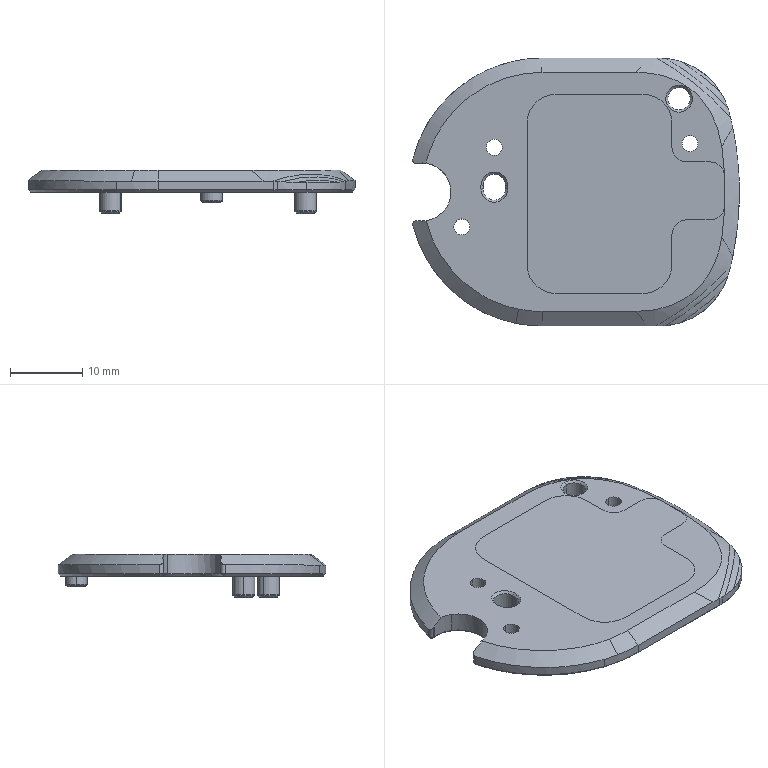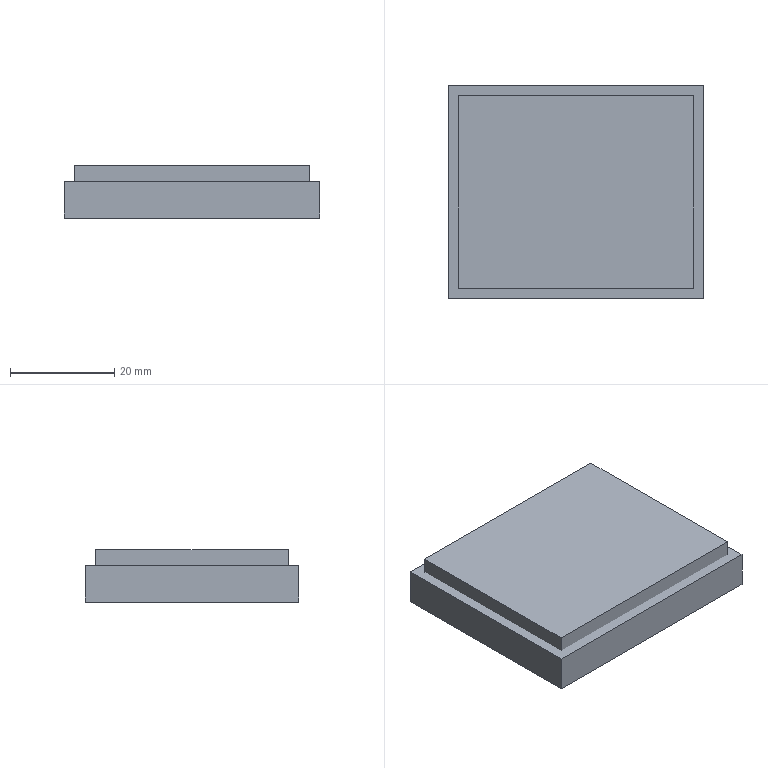CAM job | NX | 3-axis milling | part box 45.101 x 36.973 x 6 mm | stock box 49.101 x 40.973 x 10 mm
Tools:
number,name,description,diameter,corner_radius,flute_length,length,flutes
19,D80,Milling Tool-5 Parameters,80.0,0.0,50.0,75.0,2
1,D6A45,Milling Tool-5 Parameters,6.0,0.0,50.0,75.0,2
15,D10,Milling Tool-5 Parameters,10.0,0.0,50.0,75.0,2
12,D6,Milling Tool-5 Parameters,6.0,0.0,50.0,75.0,2
16,D1.5,Milling Tool-5 Parameters,1.5,0.0,50.0,75.0,2
17,D2,Milling Tool-5 Parameters,2.0,0.0,50.0,75.0,2
18,D3R0.5,Milling Tool-5 Parameters,3.0,0.5,50.0,75.0,2
11,D4,Milling Tool-5 Parameters,4.0,0.0,50.0,75.0,2
Operations:
program,operation,operation_type,tool,method,geometry_group,spindle_rpm,surface_speed,feed_per_tooth,feed_cut,feed_plunge,cut_length_mm,path_length_mm,cut_time_min,machine_time_min
1,FLOOR_WALL_COPY,VolumeBased25DMillingOperation,D80,METHOD,A,6500.0,1633.0,0.1154,1500.0,100.0,145.101,199.101,0.0967,0.1021
1,ZLEVEL_PROFILE,ZLevelMilling,D10,METHOD,A,9500.0,298.0,0.1684,3200.0,1000.0,1139.42,1202.42,0.3889,0.3952
1,CAVITY_MILL_COPY,CavityMilling,D6,METHOD,A,9509.0,179.0,0.0946,1800.0,1000.0,147.24,243.225,0.0939,0.1035
1,ZLEVEL_PROFILE_1_COPY_COPY_1,ZLevelMilling,D6,METHOD,A,9500.0,298.0,0.0658,1250.0,100.0,169.751,239.752,0.1358,0.1428
1,ZLEVEL_PROFILE_COPY,ZLevelMilling,D2,METHOD,A,9500.0,59.0,0.0632,1200.0,1000.0,199.962,347.502,0.1771,0.1919
1,HOLE_MILLING,CylinderMilling,D1.5,METHOD,A,9500.0,44.0,0.0526,1000.0,100.0,117.525,343.915,0.1175,0.1402
1,ZLEVEL_PROFILE_1,ZLevelMilling,D3R0.5,METHOD,A,9500.0,119.0,0.1579,3000.0,1000.0,5373.378,5499.902,1.794,1.806
1,PLANAR_MILL,PlanarMilling,D6A45,METHOD,A,9500.0,179.0,0.0658,1250.0,100.0,48.198,255.386,0.0386,0.0593
1,PLANAR_MILL_COPY,PlanarMilling,D6A45,METHOD,A,9500.0,179.0,0.0658,1250.0,100.0,42.168,183.826,0.0337,0.0479
1,刀补,ZLevelMilling,D2,METHOD,A,9500.0,59.0,0.0526,1000.0,1000.0,33.997,186.22,0.034,0.0492
1,刀补16,CylinderMilling,D1.5,METHOD,A,9500.0,44.0,0.0526,1000.0,100.0,30.758,257.149,0.0308,0.0534
2,FLOOR_WALL_COPY_COPY,VolumeBased25DMillingOperation,D80,METHOD,B,6500.0,1633.0,0.1154,1500.0,100.0,564.403,1173.706,0.3763,0.4372
2,CAVITY_MILL,CavityMilling,D6,METHOD,B,9500.0,298.0,0.1579,3000.0,1000.0,6689.772,7106.483,2.47,2.512
2,FLOOR_WALL_2_COPY_COPY,VolumeBased25DMillingOperation,D4,METHOD,B,9500.0,298.0,0.0658,1250.0,100.0,921.849,1351.144,0.7375,0.7804
2,CAVITY_MILL_COPY_COPY,CavityMilling,D4,METHOD,B,9500.0,119.0,0.0789,1500.0,1000.0,177.261,499.282,0.1376,0.1698
2,ZLEVEL_PROFILE_1_COPY_COPY_1_COPY,ZLevelMilling,D4,METHOD,B,9500.0,298.0,0.0658,1250.0,100.0,91.577,161.577,0.0733,0.0803
2,HOLE_MILLING_1,CylinderMilling,D2,METHOD,B,9500.0,59.0,0.0658,1250.0,100.0,209.797,456.215,0.1678,0.1925
2,ZLEVEL_PROFILE_1_COPY,ZLevelMilling,D3R0.5,METHOD,B,9500.0,119.0,0.1579,3000.0,1000.0,280.454,345.444,0.0947,0.1011
2,ZLEVEL_PROFILE_1_COPY_COPY,ZLevelMilling,D3R0.5,METHOD,B,9500.0,119.0,0.1579,3000.0,1000.0,454.68,602.293,0.1539,0.1687
2,ZLEVEL_PROFILE_1_COPY_COPY_COPY,ZLevelMilling,D3R0.5,METHOD,B,9500.0,119.0,0.1579,3000.0,1000.0,227.334,289.154,0.077,0.0831
2,FIXED_CONTOUR,SurfaceContour,D3R0.5,METHOD,B,9500.0,89.0,0.1316,2500.0,1000.0,1613.426,1672.825,0.6477,0.6537
2,PLANAR_MILL_COPY_COPY,PlanarMilling,D6A45,METHOD,B,9500.0,179.0,0.0658,1250.0,100.0,157.581,220.581,0.1261,0.1324
2,PLANAR_MILL_COPY_COPY_COPY,PlanarMilling,D6A45,METHOD,B,9500.0,179.0,0.0658,1250.0,100.0,100.751,459.606,0.0806,0.1165
2,刀补11,VolumeBased25DMillingOperation,D4,METHOD,B,9500.0,298.0,0.0658,1250.0,100.0,81.551,345.458,0.0652,0.0916